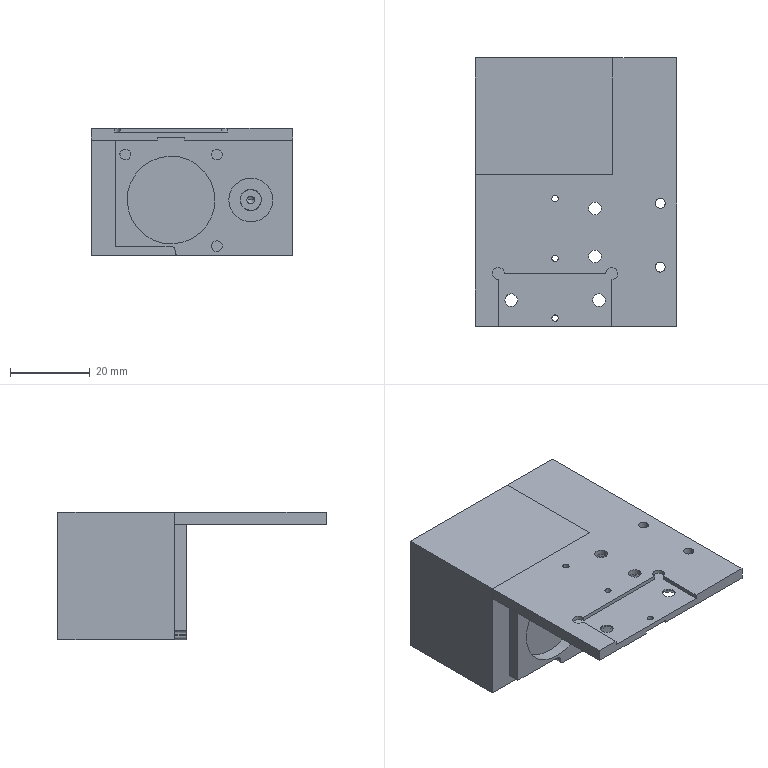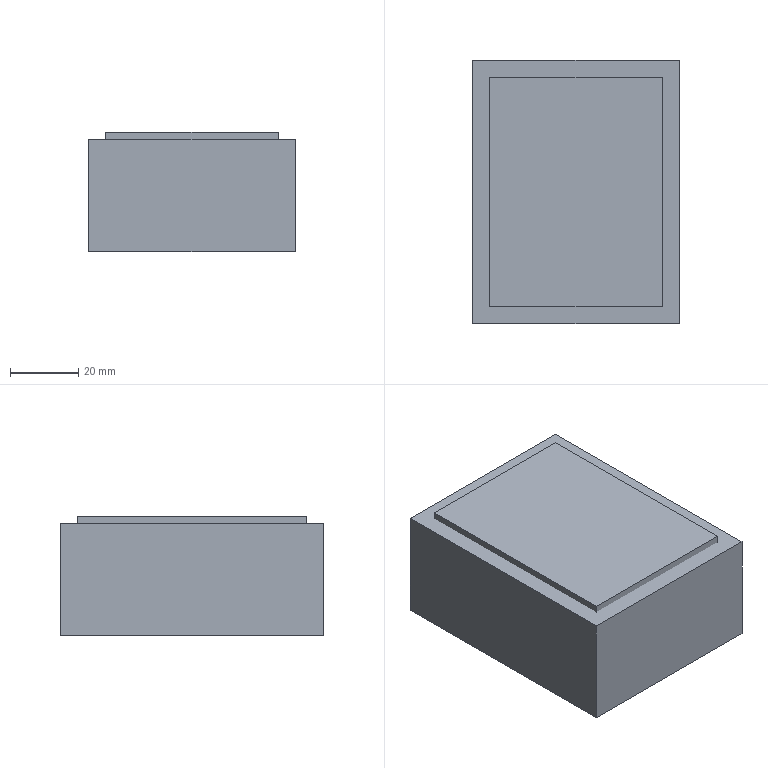CAM job | NX | 3+2 milling, drilling | part box 50.5 x 67.3 x 32 mm | stock box 60.5 x 77.3 x 35 mm
Tools:
number,name,description,diameter,corner_radius,flute_length,length,flutes
1,D63,Milling Tool-5 Parameters,63.0,0.0,50.0,75.0,2
7,D6A45,Milling Tool-5 Parameters,6.0,0.0,50.0,75.0,2
10,D10,Milling Tool-5 Parameters,10.0,0.0,50.0,75.0,2
4,D4,Milling Tool-5 Parameters,4.0,0.0,50.0,75.0,2
12,2.5ZT,Drilling Tool,2.5,0.0,35.0,50.0,2
16,1.6ZT,Drilling Tool,1.6,0.0,35.0,50.0,2
13,3.2ZT,Drilling Tool,3.2,0.0,35.0,50.0,2
2,D2,Milling Tool-5 Parameters,2.0,0.0,50.0,75.0,2
6,D6,Milling Tool-5 Parameters,6.0,0.0,50.0,75.0,2
5,D3R0.5,Milling Tool-5 Parameters,3.0,0.5,50.0,75.0,2
11,2.0ZT,Drilling Tool,1.9,0.0,35.0,50.0,2
3,D3,Milling Tool-5 Parameters,3.0,0.0,50.0,75.0,2
17,2.7ZT,Drilling Tool,2.6,0.0,35.0,50.0,2
15,5.4ZT,Drilling Tool,5.4,0.0,35.0,50.0,2
18,1.0ZT,Drilling Tool,1.0,0.0,35.0,50.0,2
23,M3,Milling Tool-5 Parameters,3.0,0.0,50.0,75.0,2
20,M2,Milling Tool-5 Parameters,1.6,0.0,50.0,75.0,2
19,UNF1-4,Milling Tool-5 Parameters,5.0,0.0,30.0,30.0,4
Operations:
program,operation,operation_type,tool,method,geometry_group,spindle_rpm,surface_speed,feed_per_tooth,feed_cut,feed_plunge,cut_length_mm,path_length_mm,cut_time_min,machine_time_min
1,FLOOR_WALL,VolumeBased25DMillingOperation,D63,METHOD,A,6500.0,1286.0,0.1154,1500.0,100.0,327.897,381.897,0.2186,0.224
1,ZLEVEL_PROFILE_3,ZLevelMilling,D10,METHOD,A,9500.0,298.0,0.1579,3000.0,1000.0,8671.445,8760.445,2.922,2.931
1,ZLEVEL_PROFILE,ZLevelMilling,D10,METHOD,A,9500.0,298.0,0.0789,1500.0,100.0,550.709,764.068,0.3671,0.3885
1,FLOOR_WALL_1_COPY_1,VolumeBased25DMillingOperation,D4,METHOD,A,9500.0,119.0,0.1316,2500.0,1000.0,630.485,827.879,0.2546,0.2744
1,FLOOR_WALL_1_COPY,VolumeBased25DMillingOperation,D4,METHOD,A,9500.0,298.0,0.0789,1500.0,1000.0,264.871,349.917,0.1784,0.1869
1,DRILLING,Operation,D6A45,METHOD,A,5000.0,94.0,0.025,250.0,0.0,36.0,262.729,0.144,0.1667
1,DRILLING_COPY,Operation,2.5ZT,METHOD,A,2000.0,15.0,0.03,120.0,0.0,15.502,110.283,0.1292,0.1387
1,DRILLING_COPY_COPY_4,Operation,M3,METHOD,A,300.0,2.0,0.0008,0.5,0.0,14.0,107.279,28.0,28.009
1,DRILLING_COPY_COPY,Operation,1.6ZT,METHOD,A,2000.0,15.0,0.03,120.0,0.0,22.442,142.705,0.187,0.199
1,DRILLING_COPY_COPY_COPY,Operation,M2,METHOD,A,300.0,1.0,0.0007,0.4,0.0,18.0,133.821,45.0,45.012
1,DRILLING_COPY_COPY_1,Operation,3.2ZT,METHOD,A,2000.0,15.0,0.03,120.0,0.0,31.846,180.011,0.2654,0.2802
1,HOLE_MILLING,CylinderMilling,D2,METHOD,A,9500.0,59.0,0.0658,1250.0,100.0,56.644,206.044,0.0453,0.0603
1,PLANAR_MILL,PlanarMilling,D6A45,METHOD,A,9500.0,179.0,0.0658,1250.0,100.0,343.288,811.466,0.2746,0.3214
1,PLANAR_MILL_COPY,PlanarMilling,D6A45,METHOD,A,9500.0,179.0,0.0658,1250.0,100.0,71.933,264.006,0.0575,0.0768
2,FLOOR_WALL_COPY,VolumeBased25DMillingOperation,D63,METHOD,B,6500.0,1286.0,0.1154,1500.0,100.0,893.691,1100.286,0.5958,0.6165
2,ADAPTIVE_MILLING_COPY,CavityMilling,D10,METHOD,B,9500.0,298.0,0.1579,3000.0,1000.0,12343.611,12829.112,5.45,5.498
2,FLOOR_WALL_1_COPY_COPY,VolumeBased25DMillingOperation,D10,METHOD,B,9500.0,298.0,0.0789,1500.0,1000.0,592.231,727.262,0.3971,0.4106
2,FLOOR_WALL_1_COPY_COPY_COPY,VolumeBased25DMillingOperation,D10,METHOD,B,9500.0,298.0,0.0789,1500.0,1000.0,125.564,380.8,0.0855,0.111
2,FLOOR_WALL_1_COPY_1_COPY,VolumeBased25DMillingOperation,D10,METHOD,B,9500.0,119.0,0.1316,2500.0,1000.0,461.539,870.645,0.1905,0.2314
2,FLOOR_WALL_1_COPY_COPY_COPY_1,VolumeBased25DMillingOperation,D10,METHOD,B,9500.0,298.0,0.0789,1500.0,1000.0,51.489,127.221,0.0365,0.0441
2,FLOOR_WALL_1_COPY_1_COPY_COPY,VolumeBased25DMillingOperation,D6,METHOD,B,9500.0,119.0,0.1316,2500.0,1000.0,2068.166,2227.541,0.8645,0.8805
2,FLOOR_WALL_1_COPY_1_COPY_COPY_COPY,VolumeBased25DMillingOperation,D6,METHOD,B,9500.0,119.0,0.0632,1200.0,1000.0,103.746,203.916,0.0869,0.097
2,FLOOR_WALL_1_COPY_1_COPY_COPY_COPY_1,VolumeBased25DMillingOperation,D6,METHOD,B,9500.0,119.0,0.0658,1250.0,1000.0,88.082,207.282,0.0708,0.0827
2,ZLEVEL_PROFILE_1,ZLevelMilling,D3R0.5,METHOD,B,9500.0,89.0,0.1316,2500.0,1000.0,148.101,207.51,0.0606,0.0666
2,DRILLING_COPY_1,Operation,D6A45,METHOD,B,5000.0,94.0,0.025,250.0,0.0,8.0,89.364,0.032,0.0401
2,DRILLING_COPY_COPY_2,Operation,2.0ZT,METHOD,B,2000.0,15.0,0.03,120.0,0.0,17.571,95.142,0.1464,0.1542
2,DRILLING_COPY_COPY_3,Operation,2.5ZT,METHOD,B,2000.0,15.0,0.03,120.0,0.0,11.251,82.502,0.0938,0.1009
2,DRILLING_COPY_COPY_4_COPY,Operation,M3,METHOD,B,300.0,2.0,0.0008,0.5,0.0,10.0,80.0,20.0,20.007
2,HOLE_MILLING_1,CylinderMilling,D3,METHOD,B,9500.0,89.0,0.0658,1250.0,100.0,273.35,342.85,0.2187,0.2256
2,DRILLING_COPY_COPY_4_COPY_COPY_1,Operation,UNF1-4,METHOD,B,300.0,4.0,0.0008,0.908,0.0,12.0,84.0,13.216,13.223
2,ZLEVEL_PROFILE_2,ZLevelMilling,D6A45,METHOD,B,9500.0,179.0,0.0658,1250.0,100.0,397.882,932.785,0.3183,0.3718
2,PLANAR_MILL_COPY_1,PlanarMilling,D6A45,METHOD,B,9500.0,179.0,0.0658,1250.0,100.0,193.556,459.426,0.1548,0.1814
2,PLANAR_MILL_COPY_1_COPY,PlanarMilling,D6A45,METHOD,B,9500.0,179.0,0.0658,1250.0,100.0,130.832,244.832,0.1047,0.1161
2,刀补6,VolumeBased25DMillingOperation,D6,METHOD,B,9500.0,119.0,0.0658,1250.0,1000.0,82.766,199.966,0.0669,0.0786
3,DRILLING_COPY_1_COPY,Operation,D6A45,METHOD,C,5000.0,94.0,0.025,250.0,0.0,17.8,235.68,0.0712,0.093
3,DRILLING_COPY_COPY_3_COPY,Operation,2.7ZT,METHOD,C,2000.0,15.0,0.03,120.0,0.0,23.343,229.076,0.1945,0.2151
3,DRILLING_COPY_COPY_3_COPY_COPY,Operation,5.4ZT,METHOD,C,2000.0,33.0,0.025,100.0,0.0,26.322,182.645,0.2632,0.2789
3,考虑铣床钻,Operation,2.0ZT,METHOD,C,2000.0,15.0,0.025,100.0,0.0,29.071,188.142,0.2907,0.3066
3,HOLE_MILLING_2,CylinderMilling,D10,METHOD,C,9500.0,298.0,0.1316,2500.0,100.0,280.527,416.527,0.1122,0.1258
3,HOLE_MILLING_2_COPY,CylinderMilling,D6,METHOD,C,9500.0,179.0,0.0789,1500.0,100.0,132.052,264.552,0.088,0.1013
3,DRILLING_COPY_COPY_4_COPY_COPY_1_COPY,Operation,UNF1-4,METHOD,C,300.0,4.0,0.0008,0.908,0.0,12.0,177.0,13.216,13.232
3,PLANAR_MILL_COPY_1_COPY_COPY,PlanarMilling,D6A45,METHOD,C,9500.0,179.0,0.0658,1250.0,100.0,273.419,1152.061,0.2187,0.3066
3,刀补10,CylinderMilling,D10,METHOD,C,9500.0,298.0,0.0789,1500.0,100.0,186.889,319.389,0.1246,0.1378
4,DRILLING_COPY_1_COPY_COPY,Operation,D6A45,METHOD,D,5000.0,94.0,0.025,250.0,0.0,14.0,133.218,0.056,0.0679
4,DRILLING_COPY_COPY_3_COPY_1,Operation,2.5ZT,METHOD,D,2000.0,15.0,0.03,120.0,0.0,35.253,168.211,0.2938,0.3071
4,DRILLING_COPY_COPY_4_COPY_COPY,Operation,M3,METHOD,D,300.0,2.0,0.0008,0.5,0.0,30.0,160.1,60.0,60.013
4,DRILLING_COPY_COPY_3_COPY_1_COPY,Operation,1.0ZT,METHOD,D,2000.0,6.0,0.02,80.0,0.0,14,88.001,0.175,0.1824
4,ZLEVEL_PROFILE_2_COPY,ZLevelMilling,D3,METHOD,D,9500.0,179.0,0.0658,1250.0,100.0,694.037,759.037,0.5552,0.5617
4,ZLEVEL_PROFILE_2_COPY_COPY,ZLevelMilling,D3,METHOD,D,9500.0,179.0,0.0658,1250.0,100.0,584.844,649.844,0.4679,0.4744
4,PLANAR_MILL_COPY_2,PlanarMilling,D6A45,METHOD,D,9500.0,179.0,0.0658,1250.0,100.0,31.934,87.434,0.0255,0.0311
5,FLOOR_WALL_1,VolumeBased25DMillingOperation,D10,METHOD,E,9500.0,298.0,0.1316,2500.0,1000.0,5122.45,5361.3,2.056,2.08
5,FLOOR_WALL_1_COPY_COPY_COPY_2,VolumeBased25DMillingOperation,D10,METHOD,E,9500.0,298.0,0.0789,1500.0,1000.0,283.106,439.532,0.1909,0.2066
5,FLOOR_WALL_1_COPY_COPY_COPY_COPY,VolumeBased25DMillingOperation,D10,METHOD,E,9500.0,298.0,0.0789,1500.0,1000.0,74.498,268.808,0.0514,0.0708
5,PLANAR_MILL_COPY_2_COPY,PlanarMilling,D6A45,METHOD,E,9500.0,179.0,0.0658,1250.0,100.0,115.731,240.731,0.0926,0.1051